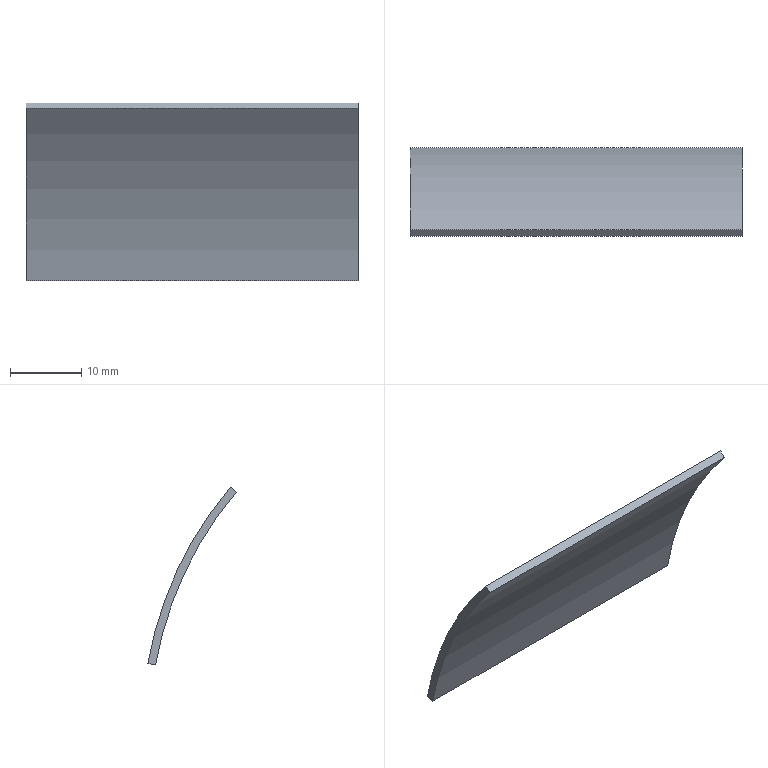Part | STEP file | basic_gh_motor_gh1_14 | 1 solid | 6 faces | box 46.5 x 12.371 x 24.915 mm | volume 1397 mm3 | plane 4 | cylinder 2 | commonest cylinder face diameters 103.2 x1 105.4 x1
STEP:
#1=CARTESIAN_POINT('',(-183.,124.399,9.151));
#2=VERTEX_POINT('',#1);
#3=CARTESIAN_POINT('',(-183.,112.871,33.875));
#4=VERTEX_POINT('',#3);
#5=CARTESIAN_POINT('',(-183.,72.5,0.));
#6=DIRECTION('',(1.,0.,0.));
#7=DIRECTION('',(0.,0.,1.));
#8=AXIS2_PLACEMENT_3D('',#5,#6,#7);
#9=CIRCLE('',#8,52.7);
#10=EDGE_CURVE('',#2,#4,#9,.T.);
#11=ORIENTED_EDGE('',*,*,#10,.T.);
#12=CARTESIAN_POINT('',(-136.5,112.871,33.875));
#13=VERTEX_POINT('',#12);
#14=CARTESIAN_POINT('',(-136.5,112.871,33.875));
#15=DIRECTION('',(-1.,0.,0.));
#16=VECTOR('',#15,1.);
#17=LINE('',#14,#16);
#18=EDGE_CURVE('',#13,#4,#17,.T.);
#19=ORIENTED_EDGE('',*,*,#18,.F.);
#20=CARTESIAN_POINT('',(-136.5,124.399,9.151));
#21=VERTEX_POINT('',#20);
#22=CARTESIAN_POINT('',(-136.5,72.5,0.));
#23=DIRECTION('',(-1.,0.,0.));
#24=DIRECTION('',(0.,0.,1.));
#25=AXIS2_PLACEMENT_3D('',#22,#23,#24);
#26=CIRCLE('',#25,52.7);
#27=EDGE_CURVE('',#13,#21,#26,.T.);
#28=ORIENTED_EDGE('',*,*,#27,.T.);
#29=CARTESIAN_POINT('',(-136.5,124.399,9.151));
#30=DIRECTION('',(-1.,0.,0.));
#31=VECTOR('',#30,1.);
#32=LINE('',#29,#31);
#33=EDGE_CURVE('',#21,#2,#32,.T.);
#34=ORIENTED_EDGE('',*,*,#33,.T.);
#35=EDGE_LOOP('',(#11,#19,#28,#34));
#36=FACE_OUTER_BOUND('',#35,.T.);
#37=CARTESIAN_POINT('',(-136.5,72.5,0.));
#38=DIRECTION('',(-1.,0.,0.));
#39=DIRECTION('',(0.,0.,1.));
#40=AXIS2_PLACEMENT_3D('',#37,#38,#39);
#41=CYLINDRICAL_SURFACE('',#40,52.7);
#42=ADVANCED_FACE('',(#36),#41,.T.);
#43=CARTESIAN_POINT('',(-183.,112.028,33.168));
#44=VERTEX_POINT('',#43);
#45=CARTESIAN_POINT('',(-183.,112.028,33.168));
#46=DIRECTION('',(0.,-0.766,-0.6428));
#47=VECTOR('',#46,1.);
#48=LINE('',#45,#47);
#49=EDGE_CURVE('',#4,#44,#48,.T.);
#50=ORIENTED_EDGE('',*,*,#49,.T.);
#51=CARTESIAN_POINT('',(-136.5,112.028,33.168));
#52=VERTEX_POINT('',#51);
#53=CARTESIAN_POINT('',(-136.5,112.028,33.168));
#54=DIRECTION('',(-1.,0.,0.));
#55=VECTOR('',#54,1.);
#56=LINE('',#53,#55);
#57=EDGE_CURVE('',#52,#44,#56,.T.);
#58=ORIENTED_EDGE('',*,*,#57,.F.);
#59=CARTESIAN_POINT('',(-136.5,112.028,33.168));
#60=DIRECTION('',(0.,0.766,0.6428));
#61=VECTOR('',#60,1.);
#62=LINE('',#59,#61);
#63=EDGE_CURVE('',#52,#13,#62,.T.);
#64=ORIENTED_EDGE('',*,*,#63,.T.);
#65=ORIENTED_EDGE('',*,*,#18,.T.);
#66=EDGE_LOOP('',(#50,#58,#64,#65));
#67=FACE_OUTER_BOUND('',#66,.T.);
#68=CARTESIAN_POINT('',(-136.5,112.449,33.521));
#69=DIRECTION('',(0.,-0.6428,0.766));
#70=DIRECTION('',(0.,0.766,0.6428));
#71=AXIS2_PLACEMENT_3D('',#68,#69,#70);
#72=PLANE('',#71);
#73=ADVANCED_FACE('',(#67),#72,.T.);
#74=CARTESIAN_POINT('',(-183.,123.316,8.96));
#75=VERTEX_POINT('',#74);
#76=CARTESIAN_POINT('',(-183.,72.5,0.));
#77=DIRECTION('',(-1.,0.,0.));
#78=DIRECTION('',(0.,0.,1.));
#79=AXIS2_PLACEMENT_3D('',#76,#77,#78);
#80=CIRCLE('',#79,51.6);
#81=EDGE_CURVE('',#44,#75,#80,.T.);
#82=ORIENTED_EDGE('',*,*,#81,.T.);
#83=CARTESIAN_POINT('',(-136.5,123.316,8.96));
#84=VERTEX_POINT('',#83);
#85=CARTESIAN_POINT('',(-136.5,123.316,8.96));
#86=DIRECTION('',(-1.,0.,0.));
#87=VECTOR('',#86,1.);
#88=LINE('',#85,#87);
#89=EDGE_CURVE('',#84,#75,#88,.T.);
#90=ORIENTED_EDGE('',*,*,#89,.F.);
#91=CARTESIAN_POINT('',(-136.5,72.5,0.));
#92=DIRECTION('',(-1.,0.,0.));
#93=DIRECTION('',(0.,0.,1.));
#94=AXIS2_PLACEMENT_3D('',#91,#92,#93);
#95=CIRCLE('',#94,51.6);
#96=EDGE_CURVE('',#52,#84,#95,.T.);
#97=ORIENTED_EDGE('',*,*,#96,.F.);
#98=ORIENTED_EDGE('',*,*,#57,.T.);
#99=EDGE_LOOP('',(#82,#90,#97,#98));
#100=FACE_OUTER_BOUND('',#99,.T.);
#101=CARTESIAN_POINT('',(-136.5,72.5,0.));
#102=DIRECTION('',(-1.,0.,0.));
#103=DIRECTION('',(0.,0.,1.));
#104=AXIS2_PLACEMENT_3D('',#101,#102,#103);
#105=CYLINDRICAL_SURFACE('',#104,51.6);
#106=ADVANCED_FACE('',(#100),#105,.F.);
#107=CARTESIAN_POINT('',(-183.,123.316,8.96));
#108=DIRECTION('',(0.,0.9848,0.1736));
#109=VECTOR('',#108,1.);
#110=LINE('',#107,#109);
#111=EDGE_CURVE('',#75,#2,#110,.T.);
#112=ORIENTED_EDGE('',*,*,#111,.T.);
#113=ORIENTED_EDGE('',*,*,#33,.F.);
#114=CARTESIAN_POINT('',(-136.5,123.316,8.96));
#115=DIRECTION('',(0.,0.9848,0.1736));
#116=VECTOR('',#115,1.);
#117=LINE('',#114,#116);
#118=EDGE_CURVE('',#84,#21,#117,.T.);
#119=ORIENTED_EDGE('',*,*,#118,.F.);
#120=ORIENTED_EDGE('',*,*,#89,.T.);
#121=EDGE_LOOP('',(#112,#113,#119,#120));
#122=FACE_OUTER_BOUND('',#121,.T.);
#123=CARTESIAN_POINT('',(-136.5,123.858,9.056));
#124=DIRECTION('',(0.,0.1736,-0.9848));
#125=DIRECTION('',(0.,-0.9848,-0.1736));
#126=AXIS2_PLACEMENT_3D('',#123,#124,#125);
#127=PLANE('',#126);
#128=ADVANCED_FACE('',(#122),#127,.T.);
#129=ORIENTED_EDGE('',*,*,#10,.F.);
#130=ORIENTED_EDGE('',*,*,#111,.F.);
#131=ORIENTED_EDGE('',*,*,#81,.F.);
#132=ORIENTED_EDGE('',*,*,#49,.F.);
#133=EDGE_LOOP('',(#129,#130,#131,#132));
#134=FACE_OUTER_BOUND('',#133,.T.);
#135=CARTESIAN_POINT('',(-183.,119.086,21.724));
#136=DIRECTION('',(-1.,0.,0.));
#137=DIRECTION('',(0.,0.,1.));
#138=AXIS2_PLACEMENT_3D('',#135,#136,#137);
#139=PLANE('',#138);
#140=ADVANCED_FACE('',(#134),#139,.T.);
#141=ORIENTED_EDGE('',*,*,#118,.T.);
#142=ORIENTED_EDGE('',*,*,#27,.F.);
#143=ORIENTED_EDGE('',*,*,#63,.F.);
#144=ORIENTED_EDGE('',*,*,#96,.T.);
#145=EDGE_LOOP('',(#141,#142,#143,#144));
#146=FACE_OUTER_BOUND('',#145,.T.);
#147=CARTESIAN_POINT('',(-136.5,119.086,21.724));
#148=DIRECTION('',(-1.,0.,0.));
#149=DIRECTION('',(0.,0.,1.));
#150=AXIS2_PLACEMENT_3D('',#147,#148,#149);
#151=PLANE('',#150);
#152=ADVANCED_FACE('',(#146),#151,.F.);
#153=CLOSED_SHELL('',(#42,#73,#106,#128,#140,#152));
#154=MANIFOLD_SOLID_BREP('',#153);
#155=(LENGTH_UNIT()NAMED_UNIT(*)SI_UNIT(.MILLI.,.METRE.));
#156=UNCERTAINTY_MEASURE_WITH_UNIT(LENGTH_MEASURE(0.01),#155,'','');
#157=(NAMED_UNIT(*)PLANE_ANGLE_UNIT()SI_UNIT($,.RADIAN.));
#158=(NAMED_UNIT(*)SI_UNIT($,.STERADIAN.)SOLID_ANGLE_UNIT());
#159=(GEOMETRIC_REPRESENTATION_CONTEXT(3)GLOBAL_UNCERTAINTY_ASSIGNED_CONTEXT((#156))GLOBAL_UNIT_ASSIGNED_CONTEXT((#155,#157,#158))REPRESENTATION_CONTEXT('',''));
#160=ADVANCED_BREP_SHAPE_REPRESENTATION('',(#154),#159);